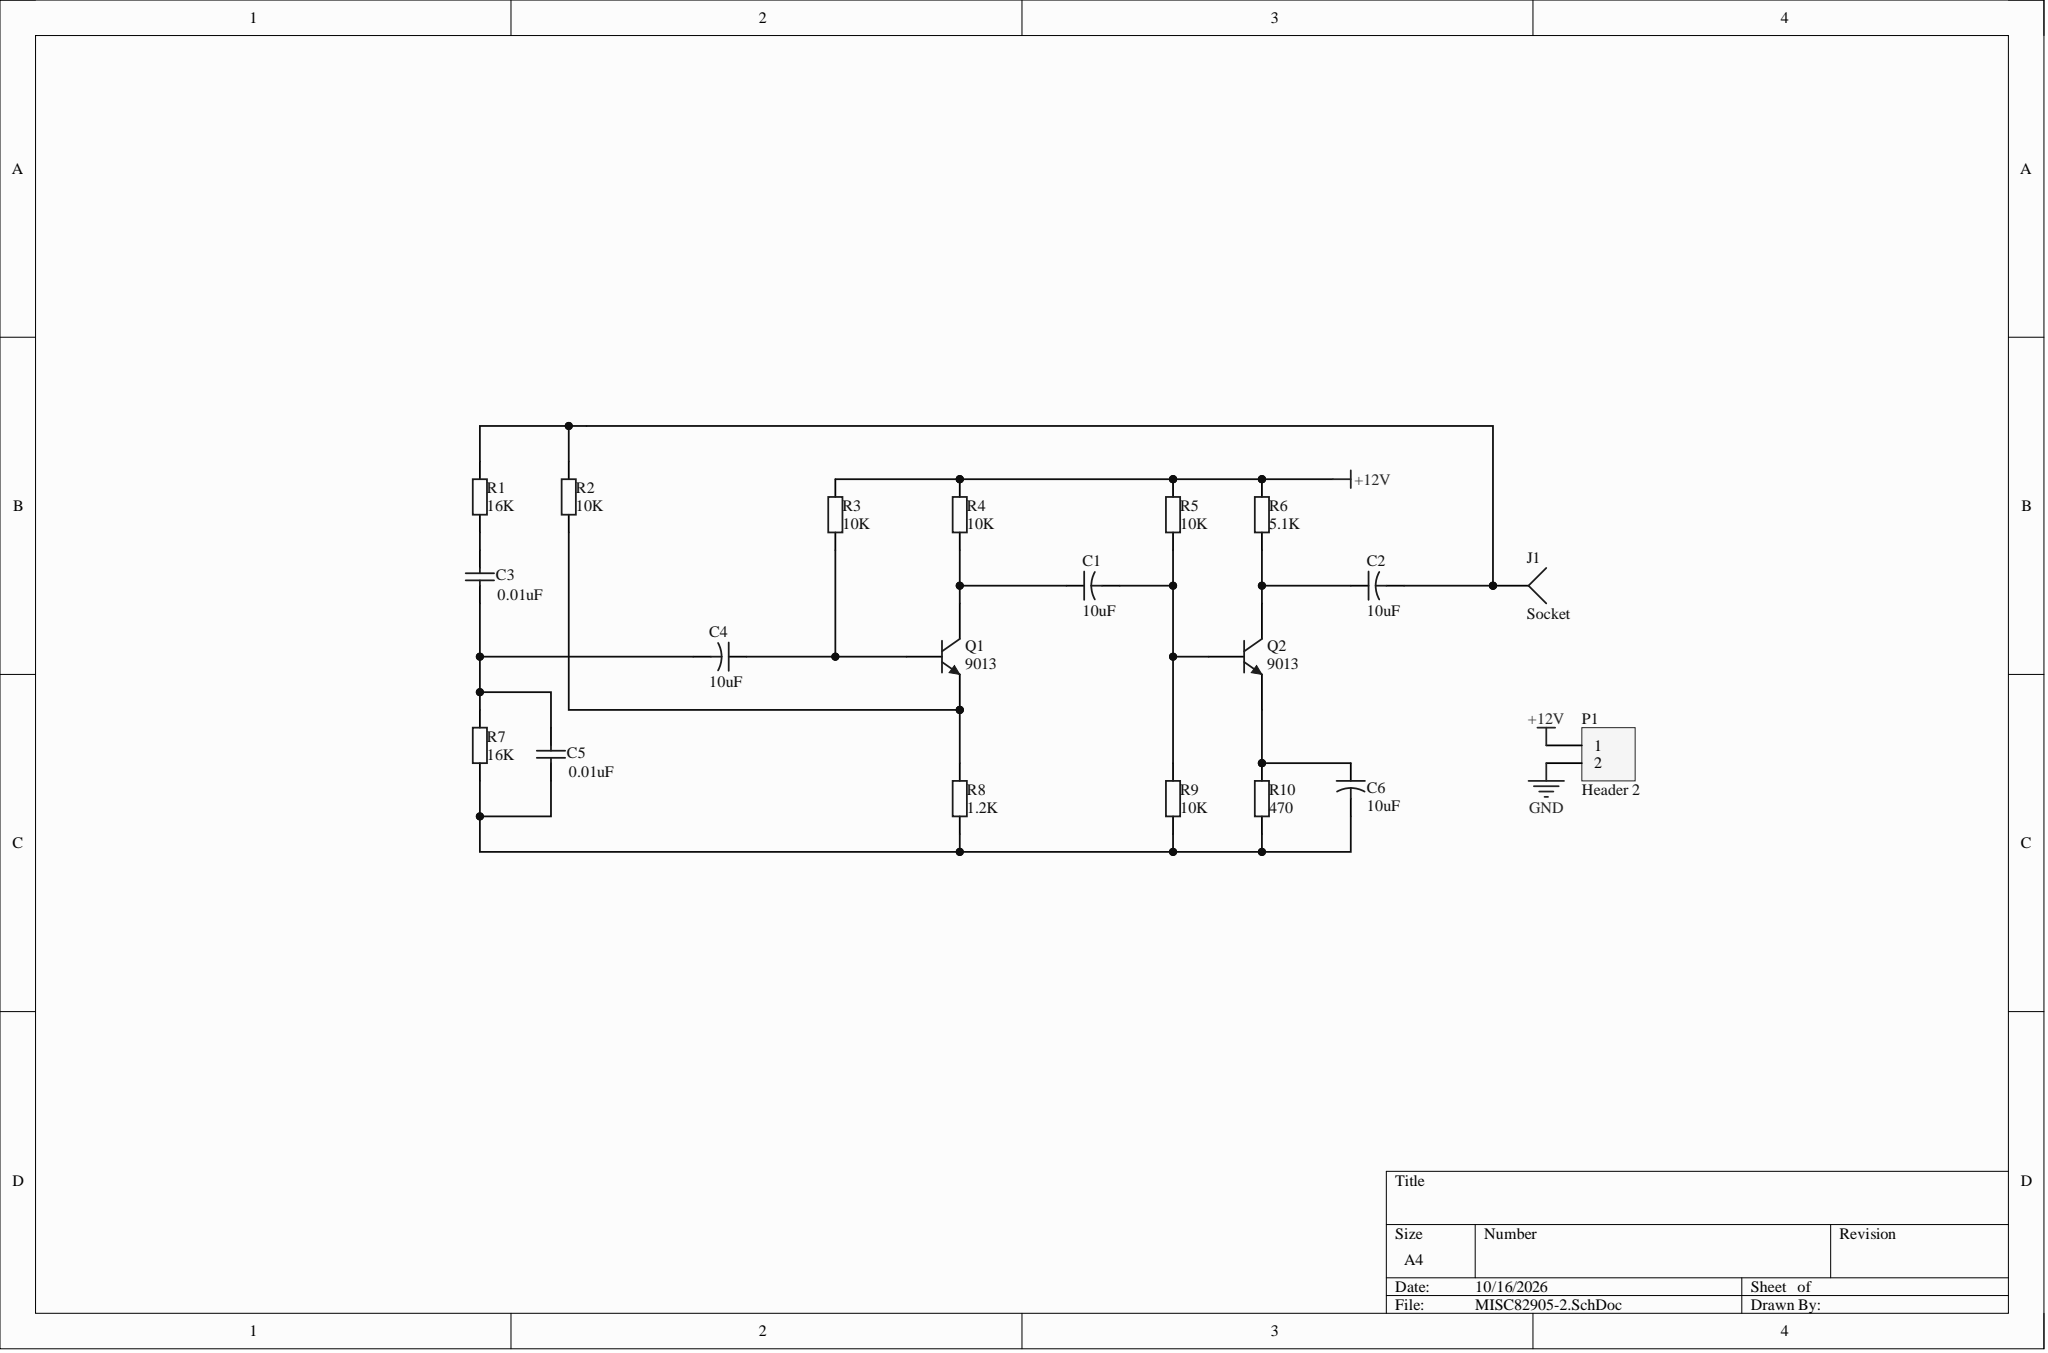Circuit board | Altium Designer | 20 parts | 11 nets
Bill of materials:
Comment,Description,Designator,Footprint,LibRef,Quantity
"10uF","Capacitor","C1, C2, C4, C6","CAPR5-4X5","Cap2","4"
"0.01uF","Capacitor","C3, C5","RAD-0.3","Cap","2"
"Socket","Socket","J1","PIN1","Socket","1"
"Header 2","Header, 2-Pin","P1","HDR1X2","Header 2","1"
"9013","NPN General Purpose Amplifier","Q1, Q2","TO-92A","2N3904","2"
"16K","Resistor","R1, R7","AXIAL-0.4","Res2","2"
"10K","Resistor","R2, R3, R4, R5, R9","AXIAL-0.4","Res2","5"
"5.1K","Resistor","R6","AXIAL-0.4","Res2","1"
"1.2K","Resistor","R8","AXIAL-0.4","Res2","1"
"470","Resistor","R10","AXIAL-0.4","Res2","1"
Netlist (Protel format):
[
C1
CAPR5-4X5
10uF



]
[
C2
CAPR5-4X5
10uF



]
[
C3
RAD-0.3
0.01uF



]
[
C4
CAPR5-4X5
10uF



]
[
C5
RAD-0.3
0.01uF



]
[
C6
CAPR5-4X5
10uF



]
[
J1
PIN1
Socket



]
[
P1
HDR1X2
Header 2



]
[
Q1
TO-92A
9013



]
[
Q2
TO-92A
9013



]
[
R1
AXIAL-0.4
16K



]
[
R2
AXIAL-0.4
10K



]
[
R3
AXIAL-0.4
10K



]
[
R4
AXIAL-0.4
10K



]
[
R5
AXIAL-0.4
10K



]
[
R6
AXIAL-0.4
5.1K



]
[
R7
AXIAL-0.4
16K



]
[
R8
AXIAL-0.4
1.2K



]
[
R9
AXIAL-0.4
10K



]
[
R10
AXIAL-0.4
470



]
(
NetQ1_1
Q1-1
R2-1
R8-2
)
(
NetC6_1
C6-1
Q2-1
R10-2
)
(
NetC5_1
C5-1
C6-2
R7-1
R8-1
R9-1
R10-1
)
(
NetC4_1
C4-1
Q1-2
R3-1
)
(
NetC3_2
C3-2
R1-1
)
(
NetC3_1
C3-1
C4-2
C5-2
R7-2
)
(
NetC2_2
C2-2
J1-1
R1-2
R2-2
)
(
NetC2_1
C2-1
Q2-3
R6-1
)
(
NetC1_2
C1-2
Q2-2
R5-1
R9-2
)
(
NetC1_1
C1-1
Q1-3
R4-1
)
(
+12V
P1-1
R3-2
R4-2
R5-2
R6-2
)